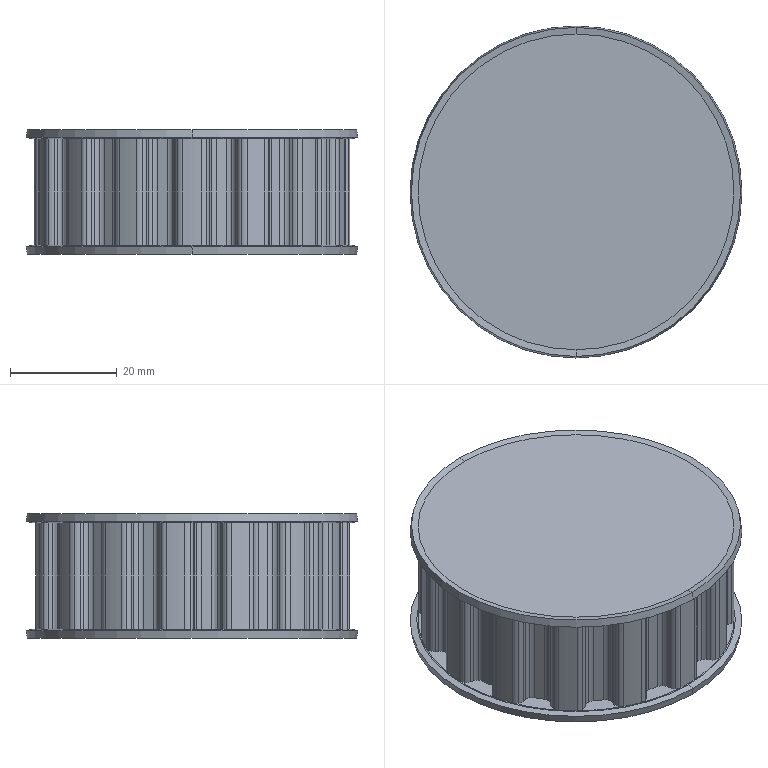Part | SolidWorks | features BaseBody 1 | 1 solid | 228 faces | box 62.266 x 62.266 x 23.437 mm | volume 59447 mm3 | cylinder 135 | plane 77 | cone 12 | torus 4 | commonest cylinder face diameters 3.2 x120 59.266 x15